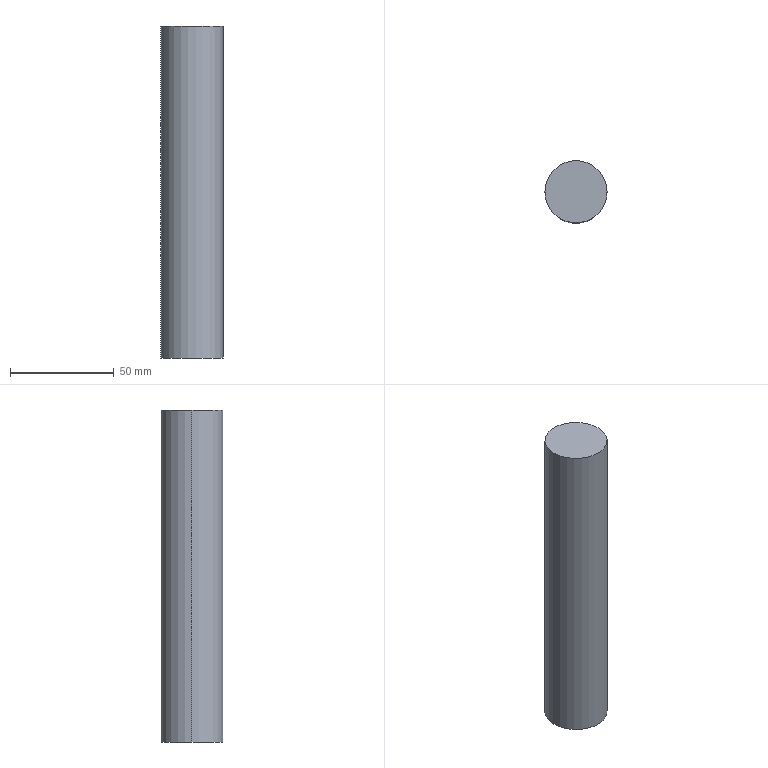Part | SolidWorks | features Extrusion 1 | 1 solid | 4 faces | box 30 x 30 x 160 mm | volume 113097 mm3 | cylinder 2 | plane 2 | commonest cylinder face diameters 30 x2
STEP:
#1=CARTESIAN_POINT('',(85.,-13.,20.));
#2=VERTEX_POINT('',#1);
#3=CARTESIAN_POINT('',(55.,-13.,20.));
#4=VERTEX_POINT('',#3);
#5=CARTESIAN_POINT('',(70.,-13.,20.));
#6=DIRECTION('',(0.,0.,1.));
#7=DIRECTION('',(1.,0.,0.));
#8=AXIS2_PLACEMENT_3D('',#5,#6,#7);
#9=CIRCLE('',#8,15.);
#10=EDGE_CURVE('',#2,#4,#9,.T.);
#11=ORIENTED_EDGE('',*,*,#10,.F.);
#12=CARTESIAN_POINT('',(85.,-13.,-140.));
#13=VERTEX_POINT('',#12);
#14=CARTESIAN_POINT('',(85.,-13.,20.));
#15=DIRECTION('',(0.,0.,-1.));
#16=VECTOR('',#15,1000.);
#17=LINE('',#14,#16);
#18=EDGE_CURVE('',#2,#13,#17,.T.);
#19=ORIENTED_EDGE('',*,*,#18,.T.);
#20=CARTESIAN_POINT('',(55.,-13.,-140.));
#21=VERTEX_POINT('',#20);
#22=CARTESIAN_POINT('',(70.,-13.,-140.));
#23=DIRECTION('',(0.,0.,1.));
#24=DIRECTION('',(1.,0.,0.));
#25=AXIS2_PLACEMENT_3D('',#22,#23,#24);
#26=CIRCLE('',#25,15.);
#27=EDGE_CURVE('',#13,#21,#26,.T.);
#28=ORIENTED_EDGE('',*,*,#27,.T.);
#29=CARTESIAN_POINT('',(55.,-13.,20.));
#30=DIRECTION('',(0.,0.,-1.));
#31=VECTOR('',#30,1000.);
#32=LINE('',#29,#31);
#33=EDGE_CURVE('',#4,#21,#32,.T.);
#34=ORIENTED_EDGE('',*,*,#33,.F.);
#35=EDGE_LOOP('',(#11,#19,#28,#34));
#36=FACE_OUTER_BOUND('',#35,.T.);
#37=CARTESIAN_POINT('',(70.,-13.,20.));
#38=DIRECTION('',(0.,0.,-1.));
#39=DIRECTION('',(-1.,0.,0.));
#40=AXIS2_PLACEMENT_3D('',#37,#38,#39);
#41=CYLINDRICAL_SURFACE('',#40,15.);
#42=ADVANCED_FACE('',(#36),#41,.T.);
#43=ORIENTED_EDGE('',*,*,#18,.F.);
#44=CARTESIAN_POINT('',(70.,-13.,20.));
#45=DIRECTION('',(0.,0.,1.));
#46=DIRECTION('',(1.,0.,0.));
#47=AXIS2_PLACEMENT_3D('',#44,#45,#46);
#48=CIRCLE('',#47,15.);
#49=EDGE_CURVE('',#4,#2,#48,.T.);
#50=ORIENTED_EDGE('',*,*,#49,.F.);
#51=ORIENTED_EDGE('',*,*,#33,.T.);
#52=CARTESIAN_POINT('',(70.,-13.,-140.));
#53=DIRECTION('',(0.,0.,1.));
#54=DIRECTION('',(1.,0.,0.));
#55=AXIS2_PLACEMENT_3D('',#52,#53,#54);
#56=CIRCLE('',#55,15.);
#57=EDGE_CURVE('',#21,#13,#56,.T.);
#58=ORIENTED_EDGE('',*,*,#57,.T.);
#59=EDGE_LOOP('',(#43,#50,#51,#58));
#60=FACE_OUTER_BOUND('',#59,.T.);
#61=CARTESIAN_POINT('',(70.,-13.,20.));
#62=DIRECTION('',(0.,0.,-1.));
#63=DIRECTION('',(-1.,0.,0.));
#64=AXIS2_PLACEMENT_3D('',#61,#62,#63);
#65=CYLINDRICAL_SURFACE('',#64,15.);
#66=ADVANCED_FACE('',(#60),#65,.T.);
#67=ORIENTED_EDGE('',*,*,#49,.T.);
#68=ORIENTED_EDGE('',*,*,#10,.T.);
#69=EDGE_LOOP('',(#67,#68));
#70=FACE_OUTER_BOUND('',#69,.T.);
#71=CARTESIAN_POINT('',(70.,-13.,20.));
#72=DIRECTION('',(0.,0.,1.));
#73=DIRECTION('',(1.,0.,0.));
#74=AXIS2_PLACEMENT_3D('',#71,#72,#73);
#75=PLANE('',#74);
#76=ADVANCED_FACE('',(#70),#75,.T.);
#77=ORIENTED_EDGE('',*,*,#57,.F.);
#78=ORIENTED_EDGE('',*,*,#27,.F.);
#79=EDGE_LOOP('',(#77,#78));
#80=FACE_OUTER_BOUND('',#79,.T.);
#81=CARTESIAN_POINT('',(70.,-13.,-140.));
#82=DIRECTION('',(0.,0.,1.));
#83=DIRECTION('',(1.,0.,0.));
#84=AXIS2_PLACEMENT_3D('',#81,#82,#83);
#85=PLANE('',#84);
#86=ADVANCED_FACE('',(#80),#85,.F.);
#87=CLOSED_SHELL('',(#42,#66,#76,#86));
#88=MANIFOLD_SOLID_BREP('',#87);
#89=CARTESIAN_POINT('',(0.,0.,0.));
#90=DIRECTION('',(0.,0.,1.));
#91=DIRECTION('',(1.,0.,0.));
#92=AXIS2_PLACEMENT_3D('',#89,#90,#91);
#93=(LENGTH_UNIT()NAMED_UNIT(*)SI_UNIT(.MILLI.,.METRE.));
#94=UNCERTAINTY_MEASURE_WITH_UNIT(LENGTH_MEASURE(0.00001),#93,'','');
#95=(NAMED_UNIT(*)PLANE_ANGLE_UNIT()SI_UNIT($,.RADIAN.));
#96=(NAMED_UNIT(*)SI_UNIT($,.STERADIAN.)SOLID_ANGLE_UNIT());
#97=(GEOMETRIC_REPRESENTATION_CONTEXT(3)GLOBAL_UNCERTAINTY_ASSIGNED_CONTEXT((#94))GLOBAL_UNIT_ASSIGNED_CONTEXT((#93,#95,#96))REPRESENTATION_CONTEXT('',''));
#98=ADVANCED_BREP_SHAPE_REPRESENTATION('',(#88,#92),#97);